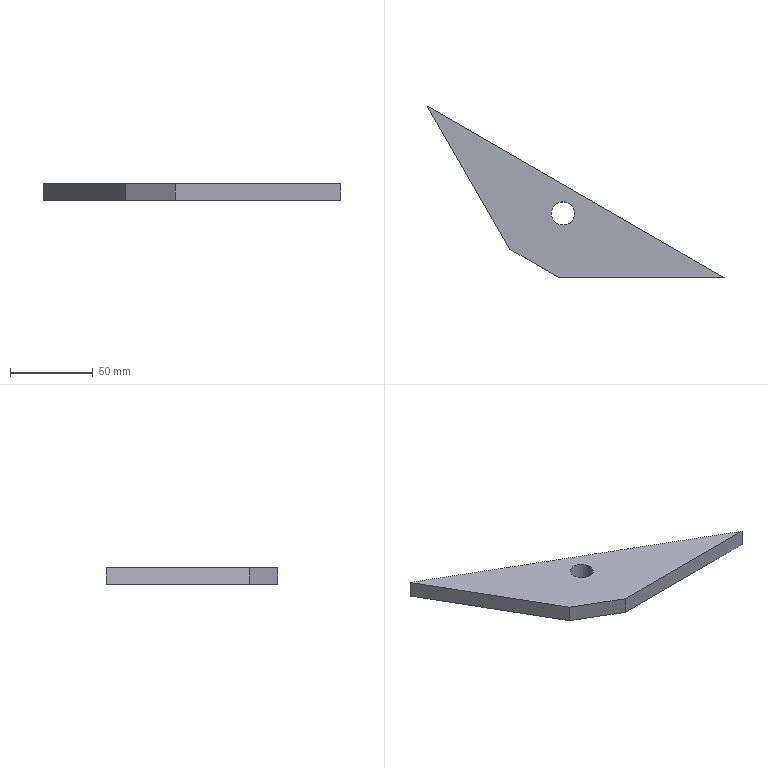Part | SolidWorks | features Extrusion 1 | 1 solid | 8 faces | box 180 x 104 x 10 mm | volume 59102 mm3 | plane 6 | cylinder 2 | commonest cylinder face diameters 14 x2
STEP:
#1=CARTESIAN_POINT('',(-5.,39.,10.));
#2=VERTEX_POINT('',#1);
#3=CARTESIAN_POINT('',(9.,39.,10.));
#4=VERTEX_POINT('',#3);
#5=CARTESIAN_POINT('',(2.,39.,10.));
#6=DIRECTION('',(0.,0.,1.));
#7=DIRECTION('',(1.,0.,0.));
#8=AXIS2_PLACEMENT_3D('',#5,#6,#7);
#9=CIRCLE('',#8,7.);
#10=EDGE_CURVE('',#2,#4,#9,.T.);
#11=ORIENTED_EDGE('',*,*,#10,.T.);
#12=CARTESIAN_POINT('',(9.,39.,0.));
#13=VERTEX_POINT('',#12);
#14=CARTESIAN_POINT('',(9.,39.,10.));
#15=DIRECTION('',(0.,0.,-1.));
#16=VECTOR('',#15,1000.);
#17=LINE('',#14,#16);
#18=EDGE_CURVE('',#4,#13,#17,.T.);
#19=ORIENTED_EDGE('',*,*,#18,.T.);
#20=CARTESIAN_POINT('',(-5.,39.,0.));
#21=VERTEX_POINT('',#20);
#22=CARTESIAN_POINT('',(2.,39.,0.));
#23=DIRECTION('',(0.,0.,1.));
#24=DIRECTION('',(1.,0.,0.));
#25=AXIS2_PLACEMENT_3D('',#22,#23,#24);
#26=CIRCLE('',#25,7.);
#27=EDGE_CURVE('',#21,#13,#26,.T.);
#28=ORIENTED_EDGE('',*,*,#27,.F.);
#29=CARTESIAN_POINT('',(-5.,39.,10.));
#30=DIRECTION('',(0.,0.,-1.));
#31=VECTOR('',#30,1000.);
#32=LINE('',#29,#31);
#33=EDGE_CURVE('',#2,#21,#32,.T.);
#34=ORIENTED_EDGE('',*,*,#33,.F.);
#35=EDGE_LOOP('',(#11,#19,#28,#34));
#36=FACE_OUTER_BOUND('',#35,.T.);
#37=CARTESIAN_POINT('',(2.,39.,10.));
#38=DIRECTION('',(0.,0.,-1.));
#39=DIRECTION('',(-1.,0.,0.));
#40=AXIS2_PLACEMENT_3D('',#37,#38,#39);
#41=CYLINDRICAL_SURFACE('',#40,7.);
#42=ADVANCED_FACE('',(#36),#41,.F.);
#43=CARTESIAN_POINT('',(100.,0.,10.));
#44=VERTEX_POINT('',#43);
#45=CARTESIAN_POINT('',(-80.,104.,10.));
#46=VERTEX_POINT('',#45);
#47=CARTESIAN_POINT('',(100.,0.,10.));
#48=DIRECTION('',(-0.8659,0.5003,0.));
#49=VECTOR('',#48,1000.);
#50=LINE('',#47,#49);
#51=EDGE_CURVE('',#44,#46,#50,.T.);
#52=ORIENTED_EDGE('',*,*,#51,.T.);
#53=CARTESIAN_POINT('',(-30.,17.397,10.));
#54=VERTEX_POINT('',#53);
#55=CARTESIAN_POINT('',(-80.,104.,10.));
#56=DIRECTION('',(0.5,-0.866,0.));
#57=VECTOR('',#56,1000.);
#58=LINE('',#55,#57);
#59=EDGE_CURVE('',#46,#54,#58,.T.);
#60=ORIENTED_EDGE('',*,*,#59,.T.);
#61=CARTESIAN_POINT('',(0.,0.,10.));
#62=VERTEX_POINT('',#61);
#63=CARTESIAN_POINT('',(-30.,17.397,10.));
#64=DIRECTION('',(0.8651,-0.5017,0.));
#65=VECTOR('',#64,1000.);
#66=LINE('',#63,#65);
#67=EDGE_CURVE('',#54,#62,#66,.T.);
#68=ORIENTED_EDGE('',*,*,#67,.T.);
#69=CARTESIAN_POINT('',(0.,0.,10.));
#70=DIRECTION('',(1.,0.,0.));
#71=VECTOR('',#70,1000.);
#72=LINE('',#69,#71);
#73=EDGE_CURVE('',#62,#44,#72,.T.);
#74=ORIENTED_EDGE('',*,*,#73,.T.);
#75=EDGE_LOOP('',(#52,#60,#68,#74));
#76=FACE_OUTER_BOUND('',#75,.T.);
#77=ORIENTED_EDGE('',*,*,#10,.F.);
#78=CARTESIAN_POINT('',(2.,39.,10.));
#79=DIRECTION('',(0.,0.,1.));
#80=DIRECTION('',(1.,0.,0.));
#81=AXIS2_PLACEMENT_3D('',#78,#79,#80);
#82=CIRCLE('',#81,7.);
#83=EDGE_CURVE('',#4,#2,#82,.T.);
#84=ORIENTED_EDGE('',*,*,#83,.F.);
#85=EDGE_LOOP('',(#77,#84));
#86=FACE_BOUND('',#85,.T.);
#87=CARTESIAN_POINT('',(0.,0.,10.));
#88=DIRECTION('',(0.,0.,-1.));
#89=DIRECTION('',(-1.,0.,0.));
#90=AXIS2_PLACEMENT_3D('',#87,#88,#89);
#91=PLANE('',#90);
#92=ADVANCED_FACE('',(#76,#86),#91,.F.);
#93=CARTESIAN_POINT('',(100.,0.,0.));
#94=VERTEX_POINT('',#93);
#95=CARTESIAN_POINT('',(-80.,104.,0.));
#96=VERTEX_POINT('',#95);
#97=CARTESIAN_POINT('',(100.,0.,0.));
#98=DIRECTION('',(-0.8659,0.5003,0.));
#99=VECTOR('',#98,1000.);
#100=LINE('',#97,#99);
#101=EDGE_CURVE('',#94,#96,#100,.T.);
#102=ORIENTED_EDGE('',*,*,#101,.F.);
#103=CARTESIAN_POINT('',(0.,0.,0.));
#104=VERTEX_POINT('',#103);
#105=CARTESIAN_POINT('',(0.,0.,0.));
#106=DIRECTION('',(1.,0.,0.));
#107=VECTOR('',#106,1000.);
#108=LINE('',#105,#107);
#109=EDGE_CURVE('',#104,#94,#108,.T.);
#110=ORIENTED_EDGE('',*,*,#109,.F.);
#111=CARTESIAN_POINT('',(-30.,17.397,0.));
#112=VERTEX_POINT('',#111);
#113=CARTESIAN_POINT('',(-30.,17.397,0.));
#114=DIRECTION('',(0.8651,-0.5017,0.));
#115=VECTOR('',#114,1000.);
#116=LINE('',#113,#115);
#117=EDGE_CURVE('',#112,#104,#116,.T.);
#118=ORIENTED_EDGE('',*,*,#117,.F.);
#119=CARTESIAN_POINT('',(-80.,104.,0.));
#120=DIRECTION('',(0.5,-0.866,0.));
#121=VECTOR('',#120,1000.);
#122=LINE('',#119,#121);
#123=EDGE_CURVE('',#96,#112,#122,.T.);
#124=ORIENTED_EDGE('',*,*,#123,.F.);
#125=EDGE_LOOP('',(#102,#110,#118,#124));
#126=FACE_OUTER_BOUND('',#125,.T.);
#127=ORIENTED_EDGE('',*,*,#27,.T.);
#128=CARTESIAN_POINT('',(2.,39.,0.));
#129=DIRECTION('',(0.,0.,1.));
#130=DIRECTION('',(1.,0.,0.));
#131=AXIS2_PLACEMENT_3D('',#128,#129,#130);
#132=CIRCLE('',#131,7.);
#133=EDGE_CURVE('',#13,#21,#132,.T.);
#134=ORIENTED_EDGE('',*,*,#133,.T.);
#135=EDGE_LOOP('',(#127,#134));
#136=FACE_BOUND('',#135,.T.);
#137=CARTESIAN_POINT('',(0.,0.,0.));
#138=DIRECTION('',(0.,0.,-1.));
#139=DIRECTION('',(-1.,0.,0.));
#140=AXIS2_PLACEMENT_3D('',#137,#138,#139);
#141=PLANE('',#140);
#142=ADVANCED_FACE('',(#126,#136),#141,.T.);
#143=ORIENTED_EDGE('',*,*,#101,.T.);
#144=CARTESIAN_POINT('',(-80.,104.,10.));
#145=DIRECTION('',(0.,0.,-1.));
#146=VECTOR('',#145,1000.);
#147=LINE('',#144,#146);
#148=EDGE_CURVE('',#46,#96,#147,.T.);
#149=ORIENTED_EDGE('',*,*,#148,.F.);
#150=ORIENTED_EDGE('',*,*,#51,.F.);
#151=CARTESIAN_POINT('',(100.,0.,10.));
#152=DIRECTION('',(0.,0.,-1.));
#153=VECTOR('',#152,1000.);
#154=LINE('',#151,#153);
#155=EDGE_CURVE('',#44,#94,#154,.T.);
#156=ORIENTED_EDGE('',*,*,#155,.T.);
#157=EDGE_LOOP('',(#143,#149,#150,#156));
#158=FACE_OUTER_BOUND('',#157,.T.);
#159=CARTESIAN_POINT('',(100.,0.,10.));
#160=DIRECTION('',(-0.5003,-0.8659,0.));
#161=DIRECTION('',(0.8659,-0.5003,0.));
#162=AXIS2_PLACEMENT_3D('',#159,#160,#161);
#163=PLANE('',#162);
#164=ADVANCED_FACE('',(#158),#163,.F.);
#165=ORIENTED_EDGE('',*,*,#123,.T.);
#166=CARTESIAN_POINT('',(-30.,17.397,10.));
#167=DIRECTION('',(0.,0.,-1.));
#168=VECTOR('',#167,1000.);
#169=LINE('',#166,#168);
#170=EDGE_CURVE('',#54,#112,#169,.T.);
#171=ORIENTED_EDGE('',*,*,#170,.F.);
#172=ORIENTED_EDGE('',*,*,#59,.F.);
#173=ORIENTED_EDGE('',*,*,#148,.T.);
#174=EDGE_LOOP('',(#165,#171,#172,#173));
#175=FACE_OUTER_BOUND('',#174,.T.);
#176=CARTESIAN_POINT('',(-80.,104.,10.));
#177=DIRECTION('',(0.866,0.5,0.));
#178=DIRECTION('',(-0.5,0.866,0.));
#179=AXIS2_PLACEMENT_3D('',#176,#177,#178);
#180=PLANE('',#179);
#181=ADVANCED_FACE('',(#175),#180,.F.);
#182=ORIENTED_EDGE('',*,*,#117,.T.);
#183=CARTESIAN_POINT('',(0.,0.,10.));
#184=DIRECTION('',(0.,0.,-1.));
#185=VECTOR('',#184,1000.);
#186=LINE('',#183,#185);
#187=EDGE_CURVE('',#62,#104,#186,.T.);
#188=ORIENTED_EDGE('',*,*,#187,.F.);
#189=ORIENTED_EDGE('',*,*,#67,.F.);
#190=ORIENTED_EDGE('',*,*,#170,.T.);
#191=EDGE_LOOP('',(#182,#188,#189,#190));
#192=FACE_OUTER_BOUND('',#191,.T.);
#193=CARTESIAN_POINT('',(-30.,17.397,10.));
#194=DIRECTION('',(0.5017,0.8651,0.));
#195=DIRECTION('',(-0.8651,0.5017,0.));
#196=AXIS2_PLACEMENT_3D('',#193,#194,#195);
#197=PLANE('',#196);
#198=ADVANCED_FACE('',(#192),#197,.F.);
#199=ORIENTED_EDGE('',*,*,#109,.T.);
#200=ORIENTED_EDGE('',*,*,#155,.F.);
#201=ORIENTED_EDGE('',*,*,#73,.F.);
#202=ORIENTED_EDGE('',*,*,#187,.T.);
#203=EDGE_LOOP('',(#199,#200,#201,#202));
#204=FACE_OUTER_BOUND('',#203,.T.);
#205=CARTESIAN_POINT('',(0.,0.,10.));
#206=DIRECTION('',(0.,1.,0.));
#207=DIRECTION('',(-1.,0.,0.));
#208=AXIS2_PLACEMENT_3D('',#205,#206,#207);
#209=PLANE('',#208);
#210=ADVANCED_FACE('',(#204),#209,.F.);
#211=ORIENTED_EDGE('',*,*,#18,.F.);
#212=ORIENTED_EDGE('',*,*,#83,.T.);
#213=ORIENTED_EDGE('',*,*,#33,.T.);
#214=ORIENTED_EDGE('',*,*,#133,.F.);
#215=EDGE_LOOP('',(#211,#212,#213,#214));
#216=FACE_OUTER_BOUND('',#215,.T.);
#217=CARTESIAN_POINT('',(2.,39.,10.));
#218=DIRECTION('',(0.,0.,-1.));
#219=DIRECTION('',(-1.,0.,0.));
#220=AXIS2_PLACEMENT_3D('',#217,#218,#219);
#221=CYLINDRICAL_SURFACE('',#220,7.);
#222=ADVANCED_FACE('',(#216),#221,.F.);
#223=CLOSED_SHELL('',(#42,#92,#142,#164,#181,#198,#210,#222));
#224=MANIFOLD_SOLID_BREP('',#223);
#225=CARTESIAN_POINT('',(0.,0.,0.));
#226=DIRECTION('',(0.,0.,1.));
#227=DIRECTION('',(1.,0.,0.));
#228=AXIS2_PLACEMENT_3D('',#225,#226,#227);
#229=(LENGTH_UNIT()NAMED_UNIT(*)SI_UNIT(.MILLI.,.METRE.));
#230=UNCERTAINTY_MEASURE_WITH_UNIT(LENGTH_MEASURE(0.00001),#229,'','');
#231=(NAMED_UNIT(*)PLANE_ANGLE_UNIT()SI_UNIT($,.RADIAN.));
#232=(NAMED_UNIT(*)SI_UNIT($,.STERADIAN.)SOLID_ANGLE_UNIT());
#233=(GEOMETRIC_REPRESENTATION_CONTEXT(3)GLOBAL_UNCERTAINTY_ASSIGNED_CONTEXT((#230))GLOBAL_UNIT_ASSIGNED_CONTEXT((#229,#231,#232))REPRESENTATION_CONTEXT('',''));
#234=ADVANCED_BREP_SHAPE_REPRESENTATION('',(#224,#228),#233);